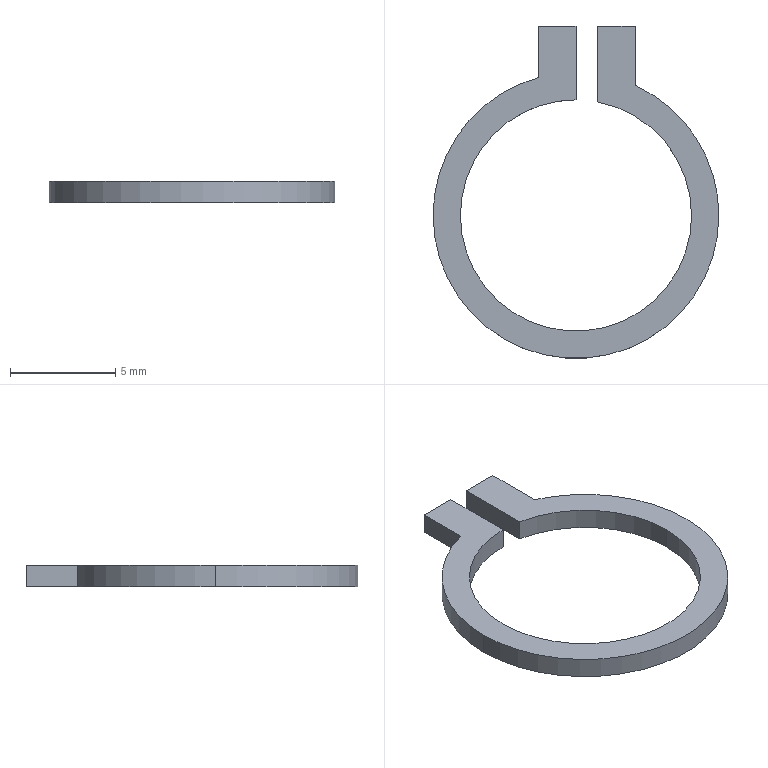Part | SolidWorks | features Extrusion 1 | 1 solid | 14 faces | box 13.6 x 15.815 x 1 mm | volume 57.5 mm3 | plane 8 | cylinder 6 | commonest cylinder face diameters 11 x3 13.6 x3
STEP:
#1=CARTESIAN_POINT('',(6.8,0.,1.));
#2=VERTEX_POINT('',#1);
#3=CARTESIAN_POINT('',(2.817,6.189,1.));
#4=VERTEX_POINT('',#3);
#5=CARTESIAN_POINT('',(0.,0.,1.));
#6=DIRECTION('',(0.,0.,1.));
#7=DIRECTION('',(1.,0.,0.));
#8=AXIS2_PLACEMENT_3D('',#5,#6,#7);
#9=CIRCLE('',#8,6.8);
#10=EDGE_CURVE('',#2,#4,#9,.T.);
#11=ORIENTED_EDGE('',*,*,#10,.F.);
#12=CARTESIAN_POINT('',(6.8,0.,0.));
#13=VERTEX_POINT('',#12);
#14=CARTESIAN_POINT('',(6.8,0.,1.));
#15=DIRECTION('',(0.,0.,-1.));
#16=VECTOR('',#15,1000.);
#17=LINE('',#14,#16);
#18=EDGE_CURVE('',#2,#13,#17,.T.);
#19=ORIENTED_EDGE('',*,*,#18,.T.);
#20=CARTESIAN_POINT('',(2.817,6.189,0.));
#21=VERTEX_POINT('',#20);
#22=CARTESIAN_POINT('',(0.,0.,0.));
#23=DIRECTION('',(0.,0.,1.));
#24=DIRECTION('',(1.,0.,0.));
#25=AXIS2_PLACEMENT_3D('',#22,#23,#24);
#26=CIRCLE('',#25,6.8);
#27=EDGE_CURVE('',#13,#21,#26,.T.);
#28=ORIENTED_EDGE('',*,*,#27,.T.);
#29=CARTESIAN_POINT('',(2.817,6.189,1.));
#30=DIRECTION('',(0.,0.,-1.));
#31=VECTOR('',#30,1000.);
#32=LINE('',#29,#31);
#33=EDGE_CURVE('',#4,#21,#32,.T.);
#34=ORIENTED_EDGE('',*,*,#33,.F.);
#35=EDGE_LOOP('',(#11,#19,#28,#34));
#36=FACE_OUTER_BOUND('',#35,.T.);
#37=CARTESIAN_POINT('',(0.,0.,1.));
#38=DIRECTION('',(0.,0.,-1.));
#39=DIRECTION('',(-1.,0.,0.));
#40=AXIS2_PLACEMENT_3D('',#37,#38,#39);
#41=CYLINDRICAL_SURFACE('',#40,6.8);
#42=ADVANCED_FACE('',(#36),#41,.T.);
#43=ORIENTED_EDGE('',*,*,#18,.F.);
#44=CARTESIAN_POINT('',(-6.8,0.,1.));
#45=VERTEX_POINT('',#44);
#46=CARTESIAN_POINT('',(0.,0.,1.));
#47=DIRECTION('',(0.,0.,1.));
#48=DIRECTION('',(1.,0.,0.));
#49=AXIS2_PLACEMENT_3D('',#46,#47,#48);
#50=CIRCLE('',#49,6.8);
#51=EDGE_CURVE('',#45,#2,#50,.T.);
#52=ORIENTED_EDGE('',*,*,#51,.F.);
#53=CARTESIAN_POINT('',(-6.8,0.,0.));
#54=VERTEX_POINT('',#53);
#55=CARTESIAN_POINT('',(-6.8,0.,1.));
#56=DIRECTION('',(0.,0.,-1.));
#57=VECTOR('',#56,1000.);
#58=LINE('',#55,#57);
#59=EDGE_CURVE('',#45,#54,#58,.T.);
#60=ORIENTED_EDGE('',*,*,#59,.T.);
#61=CARTESIAN_POINT('',(0.,0.,0.));
#62=DIRECTION('',(0.,0.,1.));
#63=DIRECTION('',(1.,0.,0.));
#64=AXIS2_PLACEMENT_3D('',#61,#62,#63);
#65=CIRCLE('',#64,6.8);
#66=EDGE_CURVE('',#54,#13,#65,.T.);
#67=ORIENTED_EDGE('',*,*,#66,.T.);
#68=EDGE_LOOP('',(#43,#52,#60,#67));
#69=FACE_OUTER_BOUND('',#68,.T.);
#70=CARTESIAN_POINT('',(0.,0.,1.));
#71=DIRECTION('',(0.,0.,-1.));
#72=DIRECTION('',(-1.,0.,0.));
#73=AXIS2_PLACEMENT_3D('',#70,#71,#72);
#74=CYLINDRICAL_SURFACE('',#73,6.8);
#75=ADVANCED_FACE('',(#69),#74,.T.);
#76=CARTESIAN_POINT('',(5.5,0.,1.));
#77=VERTEX_POINT('',#76);
#78=CARTESIAN_POINT('',(-5.5,0.,1.));
#79=VERTEX_POINT('',#78);
#80=CARTESIAN_POINT('',(0.,0.,1.));
#81=DIRECTION('',(0.,0.,-1.));
#82=DIRECTION('',(1.,0.,0.));
#83=AXIS2_PLACEMENT_3D('',#80,#81,#82);
#84=CIRCLE('',#83,5.5);
#85=EDGE_CURVE('',#77,#79,#84,.T.);
#86=ORIENTED_EDGE('',*,*,#85,.F.);
#87=CARTESIAN_POINT('',(5.5,0.,0.));
#88=VERTEX_POINT('',#87);
#89=CARTESIAN_POINT('',(5.5,0.,1.));
#90=DIRECTION('',(0.,0.,-1.));
#91=VECTOR('',#90,1000.);
#92=LINE('',#89,#91);
#93=EDGE_CURVE('',#77,#88,#92,.T.);
#94=ORIENTED_EDGE('',*,*,#93,.T.);
#95=CARTESIAN_POINT('',(-5.5,0.,0.));
#96=VERTEX_POINT('',#95);
#97=CARTESIAN_POINT('',(0.,0.,0.));
#98=DIRECTION('',(0.,0.,-1.));
#99=DIRECTION('',(1.,0.,0.));
#100=AXIS2_PLACEMENT_3D('',#97,#98,#99);
#101=CIRCLE('',#100,5.5);
#102=EDGE_CURVE('',#88,#96,#101,.T.);
#103=ORIENTED_EDGE('',*,*,#102,.T.);
#104=CARTESIAN_POINT('',(-5.5,0.,1.));
#105=DIRECTION('',(0.,0.,-1.));
#106=VECTOR('',#105,1000.);
#107=LINE('',#104,#106);
#108=EDGE_CURVE('',#79,#96,#107,.T.);
#109=ORIENTED_EDGE('',*,*,#108,.F.);
#110=EDGE_LOOP('',(#86,#94,#103,#109));
#111=FACE_OUTER_BOUND('',#110,.T.);
#112=CARTESIAN_POINT('',(0.,0.,1.));
#113=DIRECTION('',(0.,0.,-1.));
#114=DIRECTION('',(-1.,0.,0.));
#115=AXIS2_PLACEMENT_3D('',#112,#113,#114);
#116=CYLINDRICAL_SURFACE('',#115,5.5);
#117=ADVANCED_FACE('',(#111),#116,.F.);
#118=CARTESIAN_POINT('',(0.,5.5,1.));
#119=VERTEX_POINT('',#118);
#120=CARTESIAN_POINT('',(0.,0.,1.));
#121=DIRECTION('',(0.,0.,-1.));
#122=DIRECTION('',(1.,0.,0.));
#123=AXIS2_PLACEMENT_3D('',#120,#121,#122);
#124=CIRCLE('',#123,5.5);
#125=EDGE_CURVE('',#79,#119,#124,.T.);
#126=ORIENTED_EDGE('',*,*,#125,.F.);
#127=ORIENTED_EDGE('',*,*,#108,.T.);
#128=CARTESIAN_POINT('',(0.,5.5,0.));
#129=VERTEX_POINT('',#128);
#130=CARTESIAN_POINT('',(0.,0.,0.));
#131=DIRECTION('',(0.,0.,-1.));
#132=DIRECTION('',(1.,0.,0.));
#133=AXIS2_PLACEMENT_3D('',#130,#131,#132);
#134=CIRCLE('',#133,5.5);
#135=EDGE_CURVE('',#96,#129,#134,.T.);
#136=ORIENTED_EDGE('',*,*,#135,.T.);
#137=CARTESIAN_POINT('',(0.,5.5,1.));
#138=DIRECTION('',(0.,0.,-1.));
#139=VECTOR('',#138,1000.);
#140=LINE('',#137,#139);
#141=EDGE_CURVE('',#119,#129,#140,.T.);
#142=ORIENTED_EDGE('',*,*,#141,.F.);
#143=EDGE_LOOP('',(#126,#127,#136,#142));
#144=FACE_OUTER_BOUND('',#143,.T.);
#145=CARTESIAN_POINT('',(0.,0.,1.));
#146=DIRECTION('',(0.,0.,-1.));
#147=DIRECTION('',(-1.,0.,0.));
#148=AXIS2_PLACEMENT_3D('',#145,#146,#147);
#149=CYLINDRICAL_SURFACE('',#148,5.5);
#150=ADVANCED_FACE('',(#144),#149,.F.);
#151=ORIENTED_EDGE('',*,*,#93,.F.);
#152=CARTESIAN_POINT('',(1.029,5.403,1.));
#153=VERTEX_POINT('',#152);
#154=CARTESIAN_POINT('',(0.,0.,1.));
#155=DIRECTION('',(0.,0.,-1.));
#156=DIRECTION('',(1.,0.,0.));
#157=AXIS2_PLACEMENT_3D('',#154,#155,#156);
#158=CIRCLE('',#157,5.5);
#159=EDGE_CURVE('',#153,#77,#158,.T.);
#160=ORIENTED_EDGE('',*,*,#159,.F.);
#161=CARTESIAN_POINT('',(1.029,5.403,0.));
#162=VERTEX_POINT('',#161);
#163=CARTESIAN_POINT('',(1.029,5.403,1.));
#164=DIRECTION('',(0.,0.,-1.));
#165=VECTOR('',#164,1000.);
#166=LINE('',#163,#165);
#167=EDGE_CURVE('',#153,#162,#166,.T.);
#168=ORIENTED_EDGE('',*,*,#167,.T.);
#169=CARTESIAN_POINT('',(0.,0.,0.));
#170=DIRECTION('',(0.,0.,-1.));
#171=DIRECTION('',(1.,0.,0.));
#172=AXIS2_PLACEMENT_3D('',#169,#170,#171);
#173=CIRCLE('',#172,5.5);
#174=EDGE_CURVE('',#162,#88,#173,.T.);
#175=ORIENTED_EDGE('',*,*,#174,.T.);
#176=EDGE_LOOP('',(#151,#160,#168,#175));
#177=FACE_OUTER_BOUND('',#176,.T.);
#178=CARTESIAN_POINT('',(0.,0.,1.));
#179=DIRECTION('',(0.,0.,-1.));
#180=DIRECTION('',(-1.,0.,0.));
#181=AXIS2_PLACEMENT_3D('',#178,#179,#180);
#182=CYLINDRICAL_SURFACE('',#181,5.5);
#183=ADVANCED_FACE('',(#177),#182,.F.);
#184=CARTESIAN_POINT('',(0.,9.015,0.));
#185=VERTEX_POINT('',#184);
#186=CARTESIAN_POINT('',(0.,5.5,0.));
#187=DIRECTION('',(0.,1.,0.));
#188=VECTOR('',#187,1000.);
#189=LINE('',#186,#188);
#190=EDGE_CURVE('',#129,#185,#189,.T.);
#191=ORIENTED_EDGE('',*,*,#190,.T.);
#192=CARTESIAN_POINT('',(0.,9.015,1.));
#193=VERTEX_POINT('',#192);
#194=CARTESIAN_POINT('',(0.,9.015,1.));
#195=DIRECTION('',(0.,0.,-1.));
#196=VECTOR('',#195,1000.);
#197=LINE('',#194,#196);
#198=EDGE_CURVE('',#193,#185,#197,.T.);
#199=ORIENTED_EDGE('',*,*,#198,.F.);
#200=CARTESIAN_POINT('',(0.,5.5,1.));
#201=DIRECTION('',(0.,1.,0.));
#202=VECTOR('',#201,1000.);
#203=LINE('',#200,#202);
#204=EDGE_CURVE('',#119,#193,#203,.T.);
#205=ORIENTED_EDGE('',*,*,#204,.F.);
#206=ORIENTED_EDGE('',*,*,#141,.T.);
#207=EDGE_LOOP('',(#191,#199,#205,#206));
#208=FACE_OUTER_BOUND('',#207,.T.);
#209=CARTESIAN_POINT('',(0.,5.5,1.));
#210=DIRECTION('',(-1.,0.,0.));
#211=DIRECTION('',(0.,0.,1.));
#212=AXIS2_PLACEMENT_3D('',#209,#210,#211);
#213=PLANE('',#212);
#214=ADVANCED_FACE('',(#208),#213,.F.);
#215=CARTESIAN_POINT('',(-1.793,9.015,0.));
#216=VERTEX_POINT('',#215);
#217=CARTESIAN_POINT('',(0.,9.015,0.));
#218=DIRECTION('',(-1.,0.,0.));
#219=VECTOR('',#218,1000.);
#220=LINE('',#217,#219);
#221=EDGE_CURVE('',#185,#216,#220,.T.);
#222=ORIENTED_EDGE('',*,*,#221,.T.);
#223=CARTESIAN_POINT('',(-1.793,9.015,1.));
#224=VERTEX_POINT('',#223);
#225=CARTESIAN_POINT('',(-1.793,9.015,1.));
#226=DIRECTION('',(0.,0.,-1.));
#227=VECTOR('',#226,1000.);
#228=LINE('',#225,#227);
#229=EDGE_CURVE('',#224,#216,#228,.T.);
#230=ORIENTED_EDGE('',*,*,#229,.F.);
#231=CARTESIAN_POINT('',(0.,9.015,1.));
#232=DIRECTION('',(-1.,0.,0.));
#233=VECTOR('',#232,1000.);
#234=LINE('',#231,#233);
#235=EDGE_CURVE('',#193,#224,#234,.T.);
#236=ORIENTED_EDGE('',*,*,#235,.F.);
#237=ORIENTED_EDGE('',*,*,#198,.T.);
#238=EDGE_LOOP('',(#222,#230,#236,#237));
#239=FACE_OUTER_BOUND('',#238,.T.);
#240=CARTESIAN_POINT('',(0.,9.015,1.));
#241=DIRECTION('',(0.,-1.,0.));
#242=DIRECTION('',(0.,0.,-1.));
#243=AXIS2_PLACEMENT_3D('',#240,#241,#242);
#244=PLANE('',#243);
#245=ADVANCED_FACE('',(#239),#244,.F.);
#246=CARTESIAN_POINT('',(-1.793,6.559,0.));
#247=VERTEX_POINT('',#246);
#248=CARTESIAN_POINT('',(-1.793,9.015,0.));
#249=DIRECTION('',(0.,-1.,0.));
#250=VECTOR('',#249,1000.);
#251=LINE('',#248,#250);
#252=EDGE_CURVE('',#216,#247,#251,.T.);
#253=ORIENTED_EDGE('',*,*,#252,.T.);
#254=CARTESIAN_POINT('',(-1.793,6.559,1.));
#255=VERTEX_POINT('',#254);
#256=CARTESIAN_POINT('',(-1.793,6.559,1.));
#257=DIRECTION('',(0.,0.,-1.));
#258=VECTOR('',#257,1000.);
#259=LINE('',#256,#258);
#260=EDGE_CURVE('',#255,#247,#259,.T.);
#261=ORIENTED_EDGE('',*,*,#260,.F.);
#262=CARTESIAN_POINT('',(-1.793,9.015,1.));
#263=DIRECTION('',(0.,-1.,0.));
#264=VECTOR('',#263,1000.);
#265=LINE('',#262,#264);
#266=EDGE_CURVE('',#224,#255,#265,.T.);
#267=ORIENTED_EDGE('',*,*,#266,.F.);
#268=ORIENTED_EDGE('',*,*,#229,.T.);
#269=EDGE_LOOP('',(#253,#261,#267,#268));
#270=FACE_OUTER_BOUND('',#269,.T.);
#271=CARTESIAN_POINT('',(-1.793,9.015,1.));
#272=DIRECTION('',(1.,0.,0.));
#273=DIRECTION('',(0.,0.,-1.));
#274=AXIS2_PLACEMENT_3D('',#271,#272,#273);
#275=PLANE('',#274);
#276=ADVANCED_FACE('',(#270),#275,.F.);
#277=ORIENTED_EDGE('',*,*,#59,.F.);
#278=CARTESIAN_POINT('',(0.,0.,1.));
#279=DIRECTION('',(0.,0.,1.));
#280=DIRECTION('',(1.,0.,0.));
#281=AXIS2_PLACEMENT_3D('',#278,#279,#280);
#282=CIRCLE('',#281,6.8);
#283=EDGE_CURVE('',#255,#45,#282,.T.);
#284=ORIENTED_EDGE('',*,*,#283,.F.);
#285=ORIENTED_EDGE('',*,*,#260,.T.);
#286=CARTESIAN_POINT('',(0.,0.,0.));
#287=DIRECTION('',(0.,0.,1.));
#288=DIRECTION('',(1.,0.,0.));
#289=AXIS2_PLACEMENT_3D('',#286,#287,#288);
#290=CIRCLE('',#289,6.8);
#291=EDGE_CURVE('',#247,#54,#290,.T.);
#292=ORIENTED_EDGE('',*,*,#291,.T.);
#293=EDGE_LOOP('',(#277,#284,#285,#292));
#294=FACE_OUTER_BOUND('',#293,.T.);
#295=CARTESIAN_POINT('',(0.,0.,1.));
#296=DIRECTION('',(0.,0.,-1.));
#297=DIRECTION('',(-1.,0.,0.));
#298=AXIS2_PLACEMENT_3D('',#295,#296,#297);
#299=CYLINDRICAL_SURFACE('',#298,6.8);
#300=ADVANCED_FACE('',(#294),#299,.T.);
#301=CARTESIAN_POINT('',(2.817,9.015,0.));
#302=VERTEX_POINT('',#301);
#303=CARTESIAN_POINT('',(2.817,9.015,0.));
#304=DIRECTION('',(0.,1.,0.));
#305=VECTOR('',#304,1000.);
#306=LINE('',#303,#305);
#307=EDGE_CURVE('',#21,#302,#306,.T.);
#308=ORIENTED_EDGE('',*,*,#307,.T.);
#309=CARTESIAN_POINT('',(2.817,9.015,1.));
#310=VERTEX_POINT('',#309);
#311=CARTESIAN_POINT('',(2.817,9.015,1.));
#312=DIRECTION('',(0.,0.,-1.));
#313=VECTOR('',#312,1000.);
#314=LINE('',#311,#313);
#315=EDGE_CURVE('',#310,#302,#314,.T.);
#316=ORIENTED_EDGE('',*,*,#315,.F.);
#317=CARTESIAN_POINT('',(2.817,9.015,1.));
#318=DIRECTION('',(0.,1.,0.));
#319=VECTOR('',#318,1000.);
#320=LINE('',#317,#319);
#321=EDGE_CURVE('',#4,#310,#320,.T.);
#322=ORIENTED_EDGE('',*,*,#321,.F.);
#323=ORIENTED_EDGE('',*,*,#33,.T.);
#324=EDGE_LOOP('',(#308,#316,#322,#323));
#325=FACE_OUTER_BOUND('',#324,.T.);
#326=CARTESIAN_POINT('',(2.817,9.015,1.));
#327=DIRECTION('',(-1.,0.,0.));
#328=DIRECTION('',(0.,0.,1.));
#329=AXIS2_PLACEMENT_3D('',#326,#327,#328);
#330=PLANE('',#329);
#331=ADVANCED_FACE('',(#325),#330,.F.);
#332=CARTESIAN_POINT('',(1.029,9.015,0.));
#333=VERTEX_POINT('',#332);
#334=CARTESIAN_POINT('',(1.029,9.015,0.));
#335=DIRECTION('',(-1.,0.,0.));
#336=VECTOR('',#335,1000.);
#337=LINE('',#334,#336);
#338=EDGE_CURVE('',#302,#333,#337,.T.);
#339=ORIENTED_EDGE('',*,*,#338,.T.);
#340=CARTESIAN_POINT('',(1.029,9.015,1.));
#341=VERTEX_POINT('',#340);
#342=CARTESIAN_POINT('',(1.029,9.015,1.));
#343=DIRECTION('',(0.,0.,-1.));
#344=VECTOR('',#343,1000.);
#345=LINE('',#342,#344);
#346=EDGE_CURVE('',#341,#333,#345,.T.);
#347=ORIENTED_EDGE('',*,*,#346,.F.);
#348=CARTESIAN_POINT('',(1.029,9.015,1.));
#349=DIRECTION('',(-1.,0.,0.));
#350=VECTOR('',#349,1000.);
#351=LINE('',#348,#350);
#352=EDGE_CURVE('',#310,#341,#351,.T.);
#353=ORIENTED_EDGE('',*,*,#352,.F.);
#354=ORIENTED_EDGE('',*,*,#315,.T.);
#355=EDGE_LOOP('',(#339,#347,#353,#354));
#356=FACE_OUTER_BOUND('',#355,.T.);
#357=CARTESIAN_POINT('',(1.029,9.015,1.));
#358=DIRECTION('',(0.,-1.,0.));
#359=DIRECTION('',(0.,0.,-1.));
#360=AXIS2_PLACEMENT_3D('',#357,#358,#359);
#361=PLANE('',#360);
#362=ADVANCED_FACE('',(#356),#361,.F.);
#363=CARTESIAN_POINT('',(1.029,5.403,0.));
#364=DIRECTION('',(0.,-1.,0.));
#365=VECTOR('',#364,1000.);
#366=LINE('',#363,#365);
#367=EDGE_CURVE('',#333,#162,#366,.T.);
#368=ORIENTED_EDGE('',*,*,#367,.T.);
#369=ORIENTED_EDGE('',*,*,#167,.F.);
#370=CARTESIAN_POINT('',(1.029,5.403,1.));
#371=DIRECTION('',(0.,-1.,0.));
#372=VECTOR('',#371,1000.);
#373=LINE('',#370,#372);
#374=EDGE_CURVE('',#341,#153,#373,.T.);
#375=ORIENTED_EDGE('',*,*,#374,.F.);
#376=ORIENTED_EDGE('',*,*,#346,.T.);
#377=EDGE_LOOP('',(#368,#369,#375,#376));
#378=FACE_OUTER_BOUND('',#377,.T.);
#379=CARTESIAN_POINT('',(1.029,5.403,1.));
#380=DIRECTION('',(1.,0.,0.));
#381=DIRECTION('',(0.,0.,-1.));
#382=AXIS2_PLACEMENT_3D('',#379,#380,#381);
#383=PLANE('',#382);
#384=ADVANCED_FACE('',(#378),#383,.F.);
#385=ORIENTED_EDGE('',*,*,#159,.T.);
#386=ORIENTED_EDGE('',*,*,#85,.T.);
#387=ORIENTED_EDGE('',*,*,#125,.T.);
#388=ORIENTED_EDGE('',*,*,#204,.T.);
#389=ORIENTED_EDGE('',*,*,#235,.T.);
#390=ORIENTED_EDGE('',*,*,#266,.T.);
#391=ORIENTED_EDGE('',*,*,#283,.T.);
#392=ORIENTED_EDGE('',*,*,#51,.T.);
#393=ORIENTED_EDGE('',*,*,#10,.T.);
#394=ORIENTED_EDGE('',*,*,#321,.T.);
#395=ORIENTED_EDGE('',*,*,#352,.T.);
#396=ORIENTED_EDGE('',*,*,#374,.T.);
#397=EDGE_LOOP('',(#385,#386,#387,#388,#389,#390,#391,#392,#393,#394,#395,#396));
#398=FACE_OUTER_BOUND('',#397,.T.);
#399=CARTESIAN_POINT('',(0.,0.,1.));
#400=DIRECTION('',(0.,0.,1.));
#401=DIRECTION('',(1.,0.,0.));
#402=AXIS2_PLACEMENT_3D('',#399,#400,#401);
#403=PLANE('',#402);
#404=ADVANCED_FACE('',(#398),#403,.T.);
#405=ORIENTED_EDGE('',*,*,#174,.F.);
#406=ORIENTED_EDGE('',*,*,#367,.F.);
#407=ORIENTED_EDGE('',*,*,#338,.F.);
#408=ORIENTED_EDGE('',*,*,#307,.F.);
#409=ORIENTED_EDGE('',*,*,#27,.F.);
#410=ORIENTED_EDGE('',*,*,#66,.F.);
#411=ORIENTED_EDGE('',*,*,#291,.F.);
#412=ORIENTED_EDGE('',*,*,#252,.F.);
#413=ORIENTED_EDGE('',*,*,#221,.F.);
#414=ORIENTED_EDGE('',*,*,#190,.F.);
#415=ORIENTED_EDGE('',*,*,#135,.F.);
#416=ORIENTED_EDGE('',*,*,#102,.F.);
#417=EDGE_LOOP('',(#405,#406,#407,#408,#409,#410,#411,#412,#413,#414,#415,#416));
#418=FACE_OUTER_BOUND('',#417,.T.);
#419=CARTESIAN_POINT('',(0.,0.,0.));
#420=DIRECTION('',(0.,0.,1.));
#421=DIRECTION('',(1.,0.,0.));
#422=AXIS2_PLACEMENT_3D('',#419,#420,#421);
#423=PLANE('',#422);
#424=ADVANCED_FACE('',(#418),#423,.F.);
#425=CLOSED_SHELL('',(#42,#75,#117,#150,#183,#214,#245,#276,#300,#331,#362,#384,#404,#424));
#426=MANIFOLD_SOLID_BREP('',#425);
#427=CARTESIAN_POINT('',(0.,0.,0.));
#428=DIRECTION('',(0.,0.,1.));
#429=DIRECTION('',(1.,0.,0.));
#430=AXIS2_PLACEMENT_3D('',#427,#428,#429);
#431=(LENGTH_UNIT()NAMED_UNIT(*)SI_UNIT(.MILLI.,.METRE.));
#432=UNCERTAINTY_MEASURE_WITH_UNIT(LENGTH_MEASURE(0.00001),#431,'','');
#433=(NAMED_UNIT(*)PLANE_ANGLE_UNIT()SI_UNIT($,.RADIAN.));
#434=(NAMED_UNIT(*)SI_UNIT($,.STERADIAN.)SOLID_ANGLE_UNIT());
#435=(GEOMETRIC_REPRESENTATION_CONTEXT(3)GLOBAL_UNCERTAINTY_ASSIGNED_CONTEXT((#432))GLOBAL_UNIT_ASSIGNED_CONTEXT((#431,#433,#434))REPRESENTATION_CONTEXT('',''));
#436=ADVANCED_BREP_SHAPE_REPRESENTATION('',(#426,#430),#435);